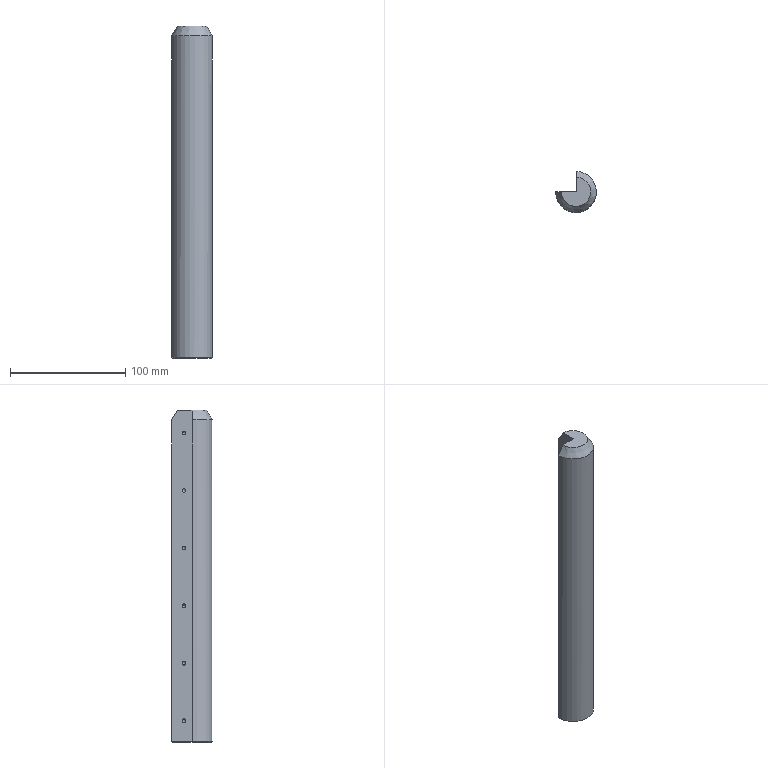Part | STEP file | Circlip fixture-large storage post | 1 solid | 34 faces | box 35.5 x 35.493 x 288.5 mm | volume 209417 mm3 | cone 15 | cylinder 13 | plane 6 | commonest cylinder face diameters 3.3 x12 35.5 x1